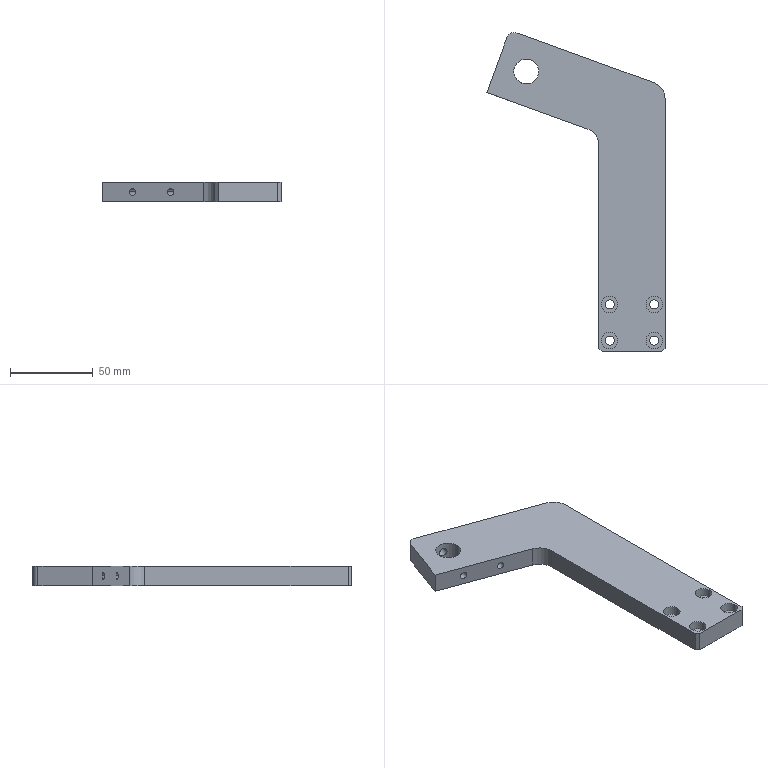Part | STEP file | 11-FG-B04911 | 1 solid | 45 faces | box 107.65 x 192.793 x 12 mm | volume 106173 mm3 | cylinder 27 | plane 14 | cone 4 | commonest cylinder face diameters 10 x9 5.5 x8 4.2 x4 5 x2 15.1 x2 20 x2
STEP:
#1=CARTESIAN_POINT('',(-47.528,162.486,6.));
#2=VERTEX_POINT('',#1);
#3=CARTESIAN_POINT('',(-43.582,161.05,6.));
#4=VERTEX_POINT('',#3);
#5=CARTESIAN_POINT('',(-45.555,161.768,6.));
#6=DIRECTION('',(-0.342,-0.9397,0.));
#7=DIRECTION('',(0.9397,-0.342,0.));
#8=AXIS2_PLACEMENT_3D('',#5,#6,#7);
#9=CIRCLE('',#8,2.1);
#10=EDGE_CURVE('',#2,#4,#9,.T.);
#11=ORIENTED_EDGE('',*,*,#10,.F.);
#12=CARTESIAN_POINT('',(-51.769,150.834,6.));
#13=VERTEX_POINT('',#12);
#14=CARTESIAN_POINT('',(-51.769,150.834,6.));
#15=DIRECTION('',(-0.342,-0.9397,0.));
#16=VECTOR('',#15,1000.);
#17=LINE('',#14,#16);
#18=EDGE_CURVE('',#2,#13,#17,.T.);
#19=ORIENTED_EDGE('',*,*,#18,.T.);
#20=CARTESIAN_POINT('',(-47.823,149.398,6.));
#21=VERTEX_POINT('',#20);
#22=CARTESIAN_POINT('',(-49.796,150.116,6.));
#23=DIRECTION('',(-0.342,-0.9397,0.));
#24=DIRECTION('',(0.9397,-0.342,0.));
#25=AXIS2_PLACEMENT_3D('',#22,#23,#24);
#26=CIRCLE('',#25,2.1);
#27=EDGE_CURVE('',#13,#21,#26,.T.);
#28=ORIENTED_EDGE('',*,*,#27,.T.);
#29=CARTESIAN_POINT('',(-47.823,149.398,6.));
#30=DIRECTION('',(-0.342,-0.9397,0.));
#31=VECTOR('',#30,1000.);
#32=LINE('',#29,#31);
#33=EDGE_CURVE('',#4,#21,#32,.T.);
#34=ORIENTED_EDGE('',*,*,#33,.F.);
#35=EDGE_LOOP('',(#11,#19,#28,#34));
#36=FACE_OUTER_BOUND('',#35,.T.);
#37=CARTESIAN_POINT('',(-49.796,150.116,6.));
#38=DIRECTION('',(-0.342,-0.9397,0.));
#39=DIRECTION('',(0.9397,-0.342,0.));
#40=AXIS2_PLACEMENT_3D('',#37,#38,#39);
#41=CYLINDRICAL_SURFACE('',#40,2.1);
#42=ADVANCED_FACE('',(#36),#41,.F.);
#43=CARTESIAN_POINT('',(-47.325,162.526,6.));
#44=VERTEX_POINT('',#43);
#45=CARTESIAN_POINT('',(-44.112,161.705,6.));
#46=VERTEX_POINT('',#45);
#47=CARTESIAN_POINT('',(-47.325,162.526,6.));
#48=CARTESIAN_POINT('',(-47.325,162.526,5.882));
#49=CARTESIAN_POINT('',(-47.317,162.522,5.765));
#50=CARTESIAN_POINT('',(-47.285,162.505,5.532));
#51=CARTESIAN_POINT('',(-47.26,162.493,5.416));
#52=CARTESIAN_POINT('',(-47.162,162.445,5.078));
#53=CARTESIAN_POINT('',(-47.065,162.398,4.868));
#54=CARTESIAN_POINT('',(-46.865,162.31,4.586));
#55=CARTESIAN_POINT('',(-46.791,162.279,4.5));
#56=CARTESIAN_POINT('',(-46.625,162.212,4.347));
#57=CARTESIAN_POINT('',(-46.532,162.177,4.278));
#58=CARTESIAN_POINT('',(-46.336,162.106,4.169));
#59=CARTESIAN_POINT('',(-46.232,162.072,4.127));
#60=CARTESIAN_POINT('',(-46.013,162.004,4.071));
#61=CARTESIAN_POINT('',(-45.898,161.971,4.058));
#62=CARTESIAN_POINT('',(-45.671,161.913,4.063));
#63=CARTESIAN_POINT('',(-45.555,161.886,4.081));
#64=CARTESIAN_POINT('',(-45.332,161.839,4.143));
#65=CARTESIAN_POINT('',(-45.223,161.819,4.188));
#66=CARTESIAN_POINT('',(-44.914,161.768,4.357));
#67=CARTESIAN_POINT('',(-44.731,161.747,4.513));
#68=CARTESIAN_POINT('',(-44.432,161.719,4.876));
#69=CARTESIAN_POINT('',(-44.313,161.713,5.086));
#70=CARTESIAN_POINT('',(-44.154,161.706,5.528));
#71=CARTESIAN_POINT('',(-44.112,161.705,5.765));
#72=CARTESIAN_POINT('',(-44.112,161.705,6.));
#73=B_SPLINE_CURVE_WITH_KNOTS('',3,(#47,#48,#49,#50,#51,#52,#53,#54,#55,#56,#57,#58,#59,#60,#61,#62,#63,#64,#65,#66,#67,#68,#69,#70,#71,#72),.UNSPECIFIED.,.F.,.F.,(4,2,2,2,2,2,2,2,2,2,2,2,4),(0.009239,0.00959,0.009941,0.01064,0.01099,0.01135,0.0117,0.01205,0.0124,0.01275,0.01345,0.01415,0.01486),.UNSPECIFIED.);
#74=EDGE_CURVE('',#44,#46,#73,.T.);
#75=ORIENTED_EDGE('',*,*,#74,.F.);
#76=CARTESIAN_POINT('',(-47.528,162.486,6.));
#77=DIRECTION('',(-0.9816,-0.1908,0.));
#78=VECTOR('',#77,1000.);
#79=LINE('',#76,#78);
#80=EDGE_CURVE('',#44,#2,#79,.T.);
#81=ORIENTED_EDGE('',*,*,#80,.T.);
#82=ORIENTED_EDGE('',*,*,#10,.T.);
#83=CARTESIAN_POINT('',(-43.582,161.05,6.));
#84=DIRECTION('',(0.6293,-0.7771,0.));
#85=VECTOR('',#84,1000.);
#86=LINE('',#83,#85);
#87=EDGE_CURVE('',#46,#4,#86,.T.);
#88=ORIENTED_EDGE('',*,*,#87,.F.);
#89=EDGE_LOOP('',(#75,#81,#82,#88));
#90=FACE_OUTER_BOUND('',#89,.T.);
#91=CARTESIAN_POINT('',(-45.555,161.768,6.));
#92=DIRECTION('',(-0.342,-0.9397,0.));
#93=DIRECTION('',(0.9397,-0.342,0.));
#94=AXIS2_PLACEMENT_3D('',#91,#92,#93);
#95=CONICAL_SURFACE('',#94,2.1,1.03);
#96=ADVANCED_FACE('',(#90),#95,.F.);
#97=CARTESIAN_POINT('',(-24.506,154.107,6.));
#98=VERTEX_POINT('',#97);
#99=CARTESIAN_POINT('',(-20.559,152.67,6.));
#100=VERTEX_POINT('',#99);
#101=CARTESIAN_POINT('',(-22.532,153.389,6.));
#102=DIRECTION('',(-0.342,-0.9397,0.));
#103=DIRECTION('',(0.9397,-0.342,0.));
#104=AXIS2_PLACEMENT_3D('',#101,#102,#103);
#105=CIRCLE('',#104,2.1);
#106=EDGE_CURVE('',#98,#100,#105,.T.);
#107=ORIENTED_EDGE('',*,*,#106,.F.);
#108=CARTESIAN_POINT('',(-28.747,142.455,6.));
#109=VERTEX_POINT('',#108);
#110=CARTESIAN_POINT('',(-28.747,142.455,6.));
#111=DIRECTION('',(-0.342,-0.9397,0.));
#112=VECTOR('',#111,1000.);
#113=LINE('',#110,#112);
#114=EDGE_CURVE('',#98,#109,#113,.T.);
#115=ORIENTED_EDGE('',*,*,#114,.T.);
#116=CARTESIAN_POINT('',(-24.8,141.018,6.));
#117=VERTEX_POINT('',#116);
#118=CARTESIAN_POINT('',(-26.773,141.736,6.));
#119=DIRECTION('',(-0.342,-0.9397,0.));
#120=DIRECTION('',(0.9397,-0.342,0.));
#121=AXIS2_PLACEMENT_3D('',#118,#119,#120);
#122=CIRCLE('',#121,2.1);
#123=EDGE_CURVE('',#109,#117,#122,.T.);
#124=ORIENTED_EDGE('',*,*,#123,.T.);
#125=CARTESIAN_POINT('',(-24.8,141.018,6.));
#126=DIRECTION('',(-0.342,-0.9397,0.));
#127=VECTOR('',#126,1000.);
#128=LINE('',#125,#127);
#129=EDGE_CURVE('',#100,#117,#128,.T.);
#130=ORIENTED_EDGE('',*,*,#129,.F.);
#131=EDGE_LOOP('',(#107,#115,#124,#130));
#132=FACE_OUTER_BOUND('',#131,.T.);
#133=CARTESIAN_POINT('',(-26.773,141.736,6.));
#134=DIRECTION('',(-0.342,-0.9397,0.));
#135=DIRECTION('',(0.9397,-0.342,0.));
#136=AXIS2_PLACEMENT_3D('',#133,#134,#135);
#137=CYLINDRICAL_SURFACE('',#136,2.1);
#138=ADVANCED_FACE('',(#132),#137,.F.);
#139=CARTESIAN_POINT('',(-22.101,154.574,6.));
#140=VERTEX_POINT('',#139);
#141=CARTESIAN_POINT('',(-20.559,152.67,6.));
#142=DIRECTION('',(0.6293,-0.7771,0.));
#143=VECTOR('',#142,1000.);
#144=LINE('',#141,#143);
#145=EDGE_CURVE('',#140,#100,#144,.T.);
#146=ORIENTED_EDGE('',*,*,#145,.F.);
#147=CARTESIAN_POINT('',(-24.506,154.107,6.));
#148=DIRECTION('',(-0.9816,-0.1908,0.));
#149=VECTOR('',#148,1000.);
#150=LINE('',#147,#149);
#151=EDGE_CURVE('',#140,#98,#150,.T.);
#152=ORIENTED_EDGE('',*,*,#151,.T.);
#153=ORIENTED_EDGE('',*,*,#106,.T.);
#154=EDGE_LOOP('',(#146,#152,#153));
#155=FACE_OUTER_BOUND('',#154,.T.);
#156=CARTESIAN_POINT('',(-22.532,153.389,6.));
#157=DIRECTION('',(-0.342,-0.9397,0.));
#158=DIRECTION('',(0.9397,-0.342,0.));
#159=AXIS2_PLACEMENT_3D('',#156,#157,#158);
#160=CONICAL_SURFACE('',#159,2.1,1.03);
#161=ADVANCED_FACE('',(#155),#160,.F.);
#162=CARTESIAN_POINT('',(-39.109,175.091,6.));
#163=VERTEX_POINT('',#162);
#164=CARTESIAN_POINT('',(-43.808,176.801,6.));
#165=VERTEX_POINT('',#164);
#166=CARTESIAN_POINT('',(-39.109,175.091,6.));
#167=CARTESIAN_POINT('',(-39.109,175.091,5.836));
#168=CARTESIAN_POINT('',(-39.123,175.102,5.671));
#169=CARTESIAN_POINT('',(-39.176,175.145,5.347));
#170=CARTESIAN_POINT('',(-39.216,175.177,5.191));
#171=CARTESIAN_POINT('',(-39.32,175.258,4.889));
#172=CARTESIAN_POINT('',(-39.385,175.307,4.743));
#173=CARTESIAN_POINT('',(-39.537,175.418,4.473));
#174=CARTESIAN_POINT('',(-39.624,175.479,4.348));
#175=CARTESIAN_POINT('',(-39.921,175.676,4.001));
#176=CARTESIAN_POINT('',(-40.159,175.82,3.818));
#177=CARTESIAN_POINT('',(-40.568,176.031,3.629));
#178=CARTESIAN_POINT('',(-40.709,176.099,3.581));
#179=CARTESIAN_POINT('',(-41.004,176.228,3.517));
#180=CARTESIAN_POINT('',(-41.158,176.29,3.5));
#181=CARTESIAN_POINT('',(-41.468,176.403,3.5));
#182=CARTESIAN_POINT('',(-41.623,176.454,3.516));
#183=CARTESIAN_POINT('',(-41.934,176.544,3.581));
#184=CARTESIAN_POINT('',(-42.089,176.584,3.629));
#185=CARTESIAN_POINT('',(-42.533,176.684,3.817));
#186=CARTESIAN_POINT('',(-42.812,176.727,4.003));
#187=CARTESIAN_POINT('',(-43.163,176.767,4.347));
#188=CARTESIAN_POINT('',(-43.271,176.777,4.475));
#189=CARTESIAN_POINT('',(-43.459,176.79,4.745));
#190=CARTESIAN_POINT('',(-43.539,176.794,4.888));
#191=CARTESIAN_POINT('',(-43.671,176.799,5.19));
#192=CARTESIAN_POINT('',(-43.722,176.8,5.349));
#193=CARTESIAN_POINT('',(-43.79,176.801,5.67));
#194=CARTESIAN_POINT('',(-43.808,176.801,5.834));
#195=CARTESIAN_POINT('',(-43.808,176.801,6.));
#196=B_SPLINE_CURVE_WITH_KNOTS('',3,(#166,#167,#168,#169,#170,#171,#172,#173,#174,#175,#176,#177,#178,#179,#180,#181,#182,#183,#184,#185,#186,#187,#188,#189,#190,#191,#192,#193,#194,#195),.UNSPECIFIED.,.F.,.F.,(4,2,2,2,2,2,2,2,2,2,2,2,2,2,4),(0.007872,0.008364,0.008856,0.009348,0.009839,0.01082,0.01131,0.01181,0.0123,0.01279,0.01377,0.01427,0.01476,0.01525,0.01574),.UNSPECIFIED.);
#197=EDGE_CURVE('',#163,#165,#196,.T.);
#198=ORIENTED_EDGE('',*,*,#197,.F.);
#199=CARTESIAN_POINT('',(-34.706,187.191,6.));
#200=VERTEX_POINT('',#199);
#201=CARTESIAN_POINT('',(-34.706,187.191,6.));
#202=DIRECTION('',(0.342,0.9397,0.));
#203=VECTOR('',#202,1000.);
#204=LINE('',#201,#203);
#205=EDGE_CURVE('',#163,#200,#204,.T.);
#206=ORIENTED_EDGE('',*,*,#205,.T.);
#207=CARTESIAN_POINT('',(-39.404,188.901,6.));
#208=VERTEX_POINT('',#207);
#209=CARTESIAN_POINT('',(-37.055,188.046,6.));
#210=DIRECTION('',(0.342,0.9397,0.));
#211=DIRECTION('',(-0.9397,0.342,0.));
#212=AXIS2_PLACEMENT_3D('',#209,#210,#211);
#213=CIRCLE('',#212,2.5);
#214=EDGE_CURVE('',#200,#208,#213,.T.);
#215=ORIENTED_EDGE('',*,*,#214,.T.);
#216=CARTESIAN_POINT('',(-39.404,188.901,6.));
#217=DIRECTION('',(0.342,0.9397,0.));
#218=VECTOR('',#217,1000.);
#219=LINE('',#216,#218);
#220=EDGE_CURVE('',#165,#208,#219,.T.);
#221=ORIENTED_EDGE('',*,*,#220,.F.);
#222=EDGE_LOOP('',(#198,#206,#215,#221));
#223=FACE_OUTER_BOUND('',#222,.T.);
#224=CARTESIAN_POINT('',(-37.055,188.046,6.));
#225=DIRECTION('',(0.342,0.9397,0.));
#226=DIRECTION('',(-0.9397,0.342,0.));
#227=AXIS2_PLACEMENT_3D('',#224,#225,#226);
#228=CYLINDRICAL_SURFACE('',#227,2.5);
#229=ADVANCED_FACE('',(#223),#228,.F.);
#230=CARTESIAN_POINT('',(1.5,28.5,6.6));
#231=VERTEX_POINT('',#230);
#232=CARTESIAN_POINT('',(11.5,28.5,6.6));
#233=VERTEX_POINT('',#232);
#234=CARTESIAN_POINT('',(6.5,28.5,6.6));
#235=DIRECTION('',(0.,0.,1.));
#236=DIRECTION('',(1.,0.,0.));
#237=AXIS2_PLACEMENT_3D('',#234,#235,#236);
#238=CIRCLE('',#237,5.);
#239=EDGE_CURVE('',#231,#233,#238,.T.);
#240=ORIENTED_EDGE('',*,*,#239,.F.);
#241=CARTESIAN_POINT('',(1.5,28.5,12.));
#242=VERTEX_POINT('',#241);
#243=CARTESIAN_POINT('',(1.5,28.5,12.));
#244=DIRECTION('',(0.,0.,1.));
#245=VECTOR('',#244,1000.);
#246=LINE('',#243,#245);
#247=EDGE_CURVE('',#231,#242,#246,.T.);
#248=ORIENTED_EDGE('',*,*,#247,.T.);
#249=CARTESIAN_POINT('',(11.5,28.5,12.));
#250=VERTEX_POINT('',#249);
#251=CARTESIAN_POINT('',(6.5,28.5,12.));
#252=DIRECTION('',(0.,0.,1.));
#253=DIRECTION('',(1.,0.,0.));
#254=AXIS2_PLACEMENT_3D('',#251,#252,#253);
#255=CIRCLE('',#254,5.);
#256=EDGE_CURVE('',#242,#250,#255,.T.);
#257=ORIENTED_EDGE('',*,*,#256,.T.);
#258=CARTESIAN_POINT('',(11.5,28.5,12.));
#259=DIRECTION('',(0.,0.,1.));
#260=VECTOR('',#259,1000.);
#261=LINE('',#258,#260);
#262=EDGE_CURVE('',#233,#250,#261,.T.);
#263=ORIENTED_EDGE('',*,*,#262,.F.);
#264=EDGE_LOOP('',(#240,#248,#257,#263));
#265=FACE_OUTER_BOUND('',#264,.T.);
#266=CARTESIAN_POINT('',(6.5,28.5,12.));
#267=DIRECTION('',(0.,0.,1.));
#268=DIRECTION('',(1.,0.,0.));
#269=AXIS2_PLACEMENT_3D('',#266,#267,#268);
#270=CYLINDRICAL_SURFACE('',#269,5.);
#271=ADVANCED_FACE('',(#265),#270,.F.);
#272=CARTESIAN_POINT('',(3.75,28.5,0.));
#273=VERTEX_POINT('',#272);
#274=CARTESIAN_POINT('',(9.25,28.5,0.));
#275=VERTEX_POINT('',#274);
#276=CARTESIAN_POINT('',(6.5,28.5,0.));
#277=DIRECTION('',(0.,0.,1.));
#278=DIRECTION('',(1.,0.,0.));
#279=AXIS2_PLACEMENT_3D('',#276,#277,#278);
#280=CIRCLE('',#279,2.75);
#281=EDGE_CURVE('',#273,#275,#280,.T.);
#282=ORIENTED_EDGE('',*,*,#281,.F.);
#283=CARTESIAN_POINT('',(3.75,28.5,6.6));
#284=VERTEX_POINT('',#283);
#285=CARTESIAN_POINT('',(3.75,28.5,12.));
#286=DIRECTION('',(0.,0.,1.));
#287=VECTOR('',#286,1000.);
#288=LINE('',#285,#287);
#289=EDGE_CURVE('',#273,#284,#288,.T.);
#290=ORIENTED_EDGE('',*,*,#289,.T.);
#291=CARTESIAN_POINT('',(9.25,28.5,6.6));
#292=VERTEX_POINT('',#291);
#293=CARTESIAN_POINT('',(6.5,28.5,6.6));
#294=DIRECTION('',(0.,0.,1.));
#295=DIRECTION('',(1.,0.,0.));
#296=AXIS2_PLACEMENT_3D('',#293,#294,#295);
#297=CIRCLE('',#296,2.75);
#298=EDGE_CURVE('',#284,#292,#297,.T.);
#299=ORIENTED_EDGE('',*,*,#298,.T.);
#300=CARTESIAN_POINT('',(9.25,28.5,12.));
#301=DIRECTION('',(0.,0.,1.));
#302=VECTOR('',#301,1000.);
#303=LINE('',#300,#302);
#304=EDGE_CURVE('',#275,#292,#303,.T.);
#305=ORIENTED_EDGE('',*,*,#304,.F.);
#306=EDGE_LOOP('',(#282,#290,#299,#305));
#307=FACE_OUTER_BOUND('',#306,.T.);
#308=CARTESIAN_POINT('',(6.5,28.5,12.));
#309=DIRECTION('',(0.,0.,1.));
#310=DIRECTION('',(1.,0.,0.));
#311=AXIS2_PLACEMENT_3D('',#308,#309,#310);
#312=CYLINDRICAL_SURFACE('',#311,2.75);
#313=ADVANCED_FACE('',(#307),#312,.F.);
#314=CARTESIAN_POINT('',(28.5,28.5,6.6));
#315=VERTEX_POINT('',#314);
#316=CARTESIAN_POINT('',(38.5,28.5,6.6));
#317=VERTEX_POINT('',#316);
#318=CARTESIAN_POINT('',(33.5,28.5,6.6));
#319=DIRECTION('',(0.,0.,1.));
#320=DIRECTION('',(1.,0.,0.));
#321=AXIS2_PLACEMENT_3D('',#318,#319,#320);
#322=CIRCLE('',#321,5.);
#323=EDGE_CURVE('',#315,#317,#322,.T.);
#324=ORIENTED_EDGE('',*,*,#323,.F.);
#325=CARTESIAN_POINT('',(28.5,28.5,12.));
#326=VERTEX_POINT('',#325);
#327=CARTESIAN_POINT('',(28.5,28.5,12.));
#328=DIRECTION('',(0.,0.,1.));
#329=VECTOR('',#328,1000.);
#330=LINE('',#327,#329);
#331=EDGE_CURVE('',#315,#326,#330,.T.);
#332=ORIENTED_EDGE('',*,*,#331,.T.);
#333=CARTESIAN_POINT('',(38.5,28.5,12.));
#334=VERTEX_POINT('',#333);
#335=CARTESIAN_POINT('',(33.5,28.5,12.));
#336=DIRECTION('',(0.,0.,1.));
#337=DIRECTION('',(1.,0.,0.));
#338=AXIS2_PLACEMENT_3D('',#335,#336,#337);
#339=CIRCLE('',#338,5.);
#340=EDGE_CURVE('',#326,#334,#339,.T.);
#341=ORIENTED_EDGE('',*,*,#340,.T.);
#342=CARTESIAN_POINT('',(38.5,28.5,12.));
#343=DIRECTION('',(0.,0.,1.));
#344=VECTOR('',#343,1000.);
#345=LINE('',#342,#344);
#346=EDGE_CURVE('',#317,#334,#345,.T.);
#347=ORIENTED_EDGE('',*,*,#346,.F.);
#348=EDGE_LOOP('',(#324,#332,#341,#347));
#349=FACE_OUTER_BOUND('',#348,.T.);
#350=CARTESIAN_POINT('',(33.5,28.5,12.));
#351=DIRECTION('',(0.,0.,1.));
#352=DIRECTION('',(1.,0.,0.));
#353=AXIS2_PLACEMENT_3D('',#350,#351,#352);
#354=CYLINDRICAL_SURFACE('',#353,5.);
#355=ADVANCED_FACE('',(#349),#354,.F.);
#356=CARTESIAN_POINT('',(30.75,28.5,0.));
#357=VERTEX_POINT('',#356);
#358=CARTESIAN_POINT('',(36.25,28.5,0.));
#359=VERTEX_POINT('',#358);
#360=CARTESIAN_POINT('',(33.5,28.5,0.));
#361=DIRECTION('',(0.,0.,1.));
#362=DIRECTION('',(1.,0.,0.));
#363=AXIS2_PLACEMENT_3D('',#360,#361,#362);
#364=CIRCLE('',#363,2.75);
#365=EDGE_CURVE('',#357,#359,#364,.T.);
#366=ORIENTED_EDGE('',*,*,#365,.F.);
#367=CARTESIAN_POINT('',(30.75,28.5,6.6));
#368=VERTEX_POINT('',#367);
#369=CARTESIAN_POINT('',(30.75,28.5,12.));
#370=DIRECTION('',(0.,0.,1.));
#371=VECTOR('',#370,1000.);
#372=LINE('',#369,#371);
#373=EDGE_CURVE('',#357,#368,#372,.T.);
#374=ORIENTED_EDGE('',*,*,#373,.T.);
#375=CARTESIAN_POINT('',(36.25,28.5,6.6));
#376=VERTEX_POINT('',#375);
#377=CARTESIAN_POINT('',(33.5,28.5,6.6));
#378=DIRECTION('',(0.,0.,1.));
#379=DIRECTION('',(1.,0.,0.));
#380=AXIS2_PLACEMENT_3D('',#377,#378,#379);
#381=CIRCLE('',#380,2.75);
#382=EDGE_CURVE('',#368,#376,#381,.T.);
#383=ORIENTED_EDGE('',*,*,#382,.T.);
#384=CARTESIAN_POINT('',(36.25,28.5,12.));
#385=DIRECTION('',(0.,0.,1.));
#386=VECTOR('',#385,1000.);
#387=LINE('',#384,#386);
#388=EDGE_CURVE('',#359,#376,#387,.T.);
#389=ORIENTED_EDGE('',*,*,#388,.F.);
#390=EDGE_LOOP('',(#366,#374,#383,#389));
#391=FACE_OUTER_BOUND('',#390,.T.);
#392=CARTESIAN_POINT('',(33.5,28.5,12.));
#393=DIRECTION('',(0.,0.,1.));
#394=DIRECTION('',(1.,0.,0.));
#395=AXIS2_PLACEMENT_3D('',#392,#393,#394);
#396=CYLINDRICAL_SURFACE('',#395,2.75);
#397=ADVANCED_FACE('',(#391),#396,.F.);
#398=CARTESIAN_POINT('',(1.5,6.5,6.6));
#399=VERTEX_POINT('',#398);
#400=CARTESIAN_POINT('',(11.5,6.5,6.6));
#401=VERTEX_POINT('',#400);
#402=CARTESIAN_POINT('',(6.5,6.5,6.6));
#403=DIRECTION('',(0.,0.,1.));
#404=DIRECTION('',(1.,0.,0.));
#405=AXIS2_PLACEMENT_3D('',#402,#403,#404);
#406=CIRCLE('',#405,5.);
#407=EDGE_CURVE('',#399,#401,#406,.T.);
#408=ORIENTED_EDGE('',*,*,#407,.F.);
#409=CARTESIAN_POINT('',(1.5,6.5,12.));
#410=VERTEX_POINT('',#409);
#411=CARTESIAN_POINT('',(1.5,6.5,12.));
#412=DIRECTION('',(0.,0.,1.));
#413=VECTOR('',#412,1000.);
#414=LINE('',#411,#413);
#415=EDGE_CURVE('',#399,#410,#414,.T.);
#416=ORIENTED_EDGE('',*,*,#415,.T.);
#417=CARTESIAN_POINT('',(11.5,6.5,12.));
#418=VERTEX_POINT('',#417);
#419=CARTESIAN_POINT('',(6.5,6.5,12.));
#420=DIRECTION('',(0.,0.,1.));
#421=DIRECTION('',(1.,0.,0.));
#422=AXIS2_PLACEMENT_3D('',#419,#420,#421);
#423=CIRCLE('',#422,5.);
#424=EDGE_CURVE('',#410,#418,#423,.T.);
#425=ORIENTED_EDGE('',*,*,#424,.T.);
#426=CARTESIAN_POINT('',(11.5,6.5,12.));
#427=DIRECTION('',(0.,0.,1.));
#428=VECTOR('',#427,1000.);
#429=LINE('',#426,#428);
#430=EDGE_CURVE('',#401,#418,#429,.T.);
#431=ORIENTED_EDGE('',*,*,#430,.F.);
#432=EDGE_LOOP('',(#408,#416,#425,#431));
#433=FACE_OUTER_BOUND('',#432,.T.);
#434=CARTESIAN_POINT('',(6.5,6.5,12.));
#435=DIRECTION('',(0.,0.,1.));
#436=DIRECTION('',(1.,0.,0.));
#437=AXIS2_PLACEMENT_3D('',#434,#435,#436);
#438=CYLINDRICAL_SURFACE('',#437,5.);
#439=ADVANCED_FACE('',(#433),#438,.F.);
#440=CARTESIAN_POINT('',(3.75,6.5,0.));
#441=VERTEX_POINT('',#440);
#442=CARTESIAN_POINT('',(9.25,6.5,0.));
#443=VERTEX_POINT('',#442);
#444=CARTESIAN_POINT('',(6.5,6.5,0.));
#445=DIRECTION('',(0.,0.,1.));
#446=DIRECTION('',(1.,0.,0.));
#447=AXIS2_PLACEMENT_3D('',#444,#445,#446);
#448=CIRCLE('',#447,2.75);
#449=EDGE_CURVE('',#441,#443,#448,.T.);
#450=ORIENTED_EDGE('',*,*,#449,.F.);
#451=CARTESIAN_POINT('',(3.75,6.5,6.6));
#452=VERTEX_POINT('',#451);
#453=CARTESIAN_POINT('',(3.75,6.5,12.));
#454=DIRECTION('',(0.,0.,1.));
#455=VECTOR('',#454,1000.);
#456=LINE('',#453,#455);
#457=EDGE_CURVE('',#441,#452,#456,.T.);
#458=ORIENTED_EDGE('',*,*,#457,.T.);
#459=CARTESIAN_POINT('',(9.25,6.5,6.6));
#460=VERTEX_POINT('',#459);
#461=CARTESIAN_POINT('',(6.5,6.5,6.6));
#462=DIRECTION('',(0.,0.,1.));
#463=DIRECTION('',(1.,0.,0.));
#464=AXIS2_PLACEMENT_3D('',#461,#462,#463);
#465=CIRCLE('',#464,2.75);
#466=EDGE_CURVE('',#452,#460,#465,.T.);
#467=ORIENTED_EDGE('',*,*,#466,.T.);
#468=CARTESIAN_POINT('',(9.25,6.5,12.));
#469=DIRECTION('',(0.,0.,1.));
#470=VECTOR('',#469,1000.);
#471=LINE('',#468,#470);
#472=EDGE_CURVE('',#443,#460,#471,.T.);
#473=ORIENTED_EDGE('',*,*,#472,.F.);
#474=EDGE_LOOP('',(#450,#458,#467,#473));
#475=FACE_OUTER_BOUND('',#474,.T.);
#476=CARTESIAN_POINT('',(6.5,6.5,12.));
#477=DIRECTION('',(0.,0.,1.));
#478=DIRECTION('',(1.,0.,0.));
#479=AXIS2_PLACEMENT_3D('',#476,#477,#478);
#480=CYLINDRICAL_SURFACE('',#479,2.75);
#481=ADVANCED_FACE('',(#475),#480,.F.);
#482=CARTESIAN_POINT('',(28.5,6.5,6.6));
#483=VERTEX_POINT('',#482);
#484=CARTESIAN_POINT('',(38.5,6.5,6.6));
#485=VERTEX_POINT('',#484);
#486=CARTESIAN_POINT('',(33.5,6.5,6.6));
#487=DIRECTION('',(0.,0.,1.));
#488=DIRECTION('',(1.,0.,0.));
#489=AXIS2_PLACEMENT_3D('',#486,#487,#488);
#490=CIRCLE('',#489,5.);
#491=EDGE_CURVE('',#483,#485,#490,.T.);
#492=ORIENTED_EDGE('',*,*,#491,.F.);
#493=CARTESIAN_POINT('',(28.5,6.5,12.));
#494=VERTEX_POINT('',#493);
#495=CARTESIAN_POINT('',(28.5,6.5,12.));
#496=DIRECTION('',(0.,0.,1.));
#497=VECTOR('',#496,1000.);
#498=LINE('',#495,#497);
#499=EDGE_CURVE('',#483,#494,#498,.T.);
#500=ORIENTED_EDGE('',*,*,#499,.T.);
#501=CARTESIAN_POINT('',(38.5,6.5,12.));
#502=VERTEX_POINT('',#501);
#503=CARTESIAN_POINT('',(33.5,6.5,12.));
#504=DIRECTION('',(0.,0.,1.));
#505=DIRECTION('',(1.,0.,0.));
#506=AXIS2_PLACEMENT_3D('',#503,#504,#505);
#507=CIRCLE('',#506,5.);
#508=EDGE_CURVE('',#494,#502,#507,.T.);
#509=ORIENTED_EDGE('',*,*,#508,.T.);
#510=CARTESIAN_POINT('',(38.5,6.5,12.));
#511=DIRECTION('',(0.,0.,1.));
#512=VECTOR('',#511,1000.);
#513=LINE('',#510,#512);
#514=EDGE_CURVE('',#485,#502,#513,.T.);
#515=ORIENTED_EDGE('',*,*,#514,.F.);
#516=EDGE_LOOP('',(#492,#500,#509,#515));
#517=FACE_OUTER_BOUND('',#516,.T.);
#518=CARTESIAN_POINT('',(33.5,6.5,12.));
#519=DIRECTION('',(0.,0.,1.));
#520=DIRECTION('',(1.,0.,0.));
#521=AXIS2_PLACEMENT_3D('',#518,#519,#520);
#522=CYLINDRICAL_SURFACE('',#521,5.);
#523=ADVANCED_FACE('',(#517),#522,.F.);
#524=CARTESIAN_POINT('',(30.75,6.5,0.));
#525=VERTEX_POINT('',#524);
#526=CARTESIAN_POINT('',(36.25,6.5,0.));
#527=VERTEX_POINT('',#526);
#528=CARTESIAN_POINT('',(33.5,6.5,0.));
#529=DIRECTION('',(0.,0.,1.));
#530=DIRECTION('',(1.,0.,0.));
#531=AXIS2_PLACEMENT_3D('',#528,#529,#530);
#532=CIRCLE('',#531,2.75);
#533=EDGE_CURVE('',#525,#527,#532,.T.);
#534=ORIENTED_EDGE('',*,*,#533,.F.);
#535=CARTESIAN_POINT('',(30.75,6.5,6.6));
#536=VERTEX_POINT('',#535);
#537=CARTESIAN_POINT('',(30.75,6.5,12.));
#538=DIRECTION('',(0.,0.,1.));
#539=VECTOR('',#538,1000.);
#540=LINE('',#537,#539);
#541=EDGE_CURVE('',#525,#536,#540,.T.);
#542=ORIENTED_EDGE('',*,*,#541,.T.);
#543=CARTESIAN_POINT('',(36.25,6.5,6.6));
#544=VERTEX_POINT('',#543);
#545=CARTESIAN_POINT('',(33.5,6.5,6.6));
#546=DIRECTION('',(0.,0.,1.));
#547=DIRECTION('',(1.,0.,0.));
#548=AXIS2_PLACEMENT_3D('',#545,#546,#547);
#549=CIRCLE('',#548,2.75);
#550=EDGE_CURVE('',#536,#544,#549,.T.);
#551=ORIENTED_EDGE('',*,*,#550,.T.);
#552=CARTESIAN_POINT('',(36.25,6.5,12.));
#553=DIRECTION('',(0.,0.,1.));
#554=VECTOR('',#553,1000.);
#555=LINE('',#552,#554);
#556=EDGE_CURVE('',#527,#544,#555,.T.);
#557=ORIENTED_EDGE('',*,*,#556,.F.);
#558=EDGE_LOOP('',(#534,#542,#551,#557));
#559=FACE_OUTER_BOUND('',#558,.T.);
#560=CARTESIAN_POINT('',(33.5,6.5,12.));
#561=DIRECTION('',(0.,0.,1.));
#562=DIRECTION('',(1.,0.,0.));
#563=AXIS2_PLACEMENT_3D('',#560,#561,#562);
#564=CYLINDRICAL_SURFACE('',#563,2.75);
#565=ADVANCED_FACE('',(#559),#564,.F.);
#566=CARTESIAN_POINT('',(-44.112,161.705,6.));
#567=CARTESIAN_POINT('',(-44.112,161.705,6.234));
#568=CARTESIAN_POINT('',(-44.154,161.706,6.472));
#569=CARTESIAN_POINT('',(-44.313,161.713,6.913));
#570=CARTESIAN_POINT('',(-44.431,161.719,7.123));
#571=CARTESIAN_POINT('',(-44.654,161.74,7.394));
#572=CARTESIAN_POINT('',(-44.738,161.748,7.479));
#573=CARTESIAN_POINT('',(-44.917,161.771,7.63));
#574=CARTESIAN_POINT('',(-45.013,161.784,7.696));
#575=CARTESIAN_POINT('',(-45.216,161.817,7.808));
#576=CARTESIAN_POINT('',(-45.325,161.838,7.854));
#577=CARTESIAN_POINT('',(-45.548,161.884,7.918));
#578=CARTESIAN_POINT('',(-45.661,161.91,7.936));
#579=CARTESIAN_POINT('',(-45.892,161.97,7.942));
#580=CARTESIAN_POINT('',(-46.005,162.002,7.93));
#581=CARTESIAN_POINT('',(-46.225,162.069,7.876));
#582=CARTESIAN_POINT('',(-46.332,162.105,7.833));
#583=CARTESIAN_POINT('',(-46.529,162.175,7.724));
#584=CARTESIAN_POINT('',(-46.621,162.211,7.657));
#585=CARTESIAN_POINT('',(-46.788,162.277,7.503));
#586=CARTESIAN_POINT('',(-46.863,162.309,7.417));
#587=CARTESIAN_POINT('',(-47.064,162.397,7.135));
#588=CARTESIAN_POINT('',(-47.162,162.445,6.922));
#589=CARTESIAN_POINT('',(-47.26,162.493,6.585));
#590=CARTESIAN_POINT('',(-47.284,162.505,6.47));
#591=CARTESIAN_POINT('',(-47.317,162.522,6.237));
#592=CARTESIAN_POINT('',(-47.325,162.526,6.118));
#593=CARTESIAN_POINT('',(-47.325,162.526,6.));
#594=B_SPLINE_CURVE_WITH_KNOTS('',3,(#566,#567,#568,#569,#570,#571,#572,#573,#574,#575,#576,#577,#578,#579,#580,#581,#582,#583,#584,#585,#586,#587,#588,#589,#590,#591,#592,#593),.UNSPECIFIED.,.F.,.F.,(4,2,2,2,2,2,2,2,2,2,2,2,2,4),(0.003628,0.004329,0.00503,0.005381,0.005732,0.006082,0.006433,0.006784,0.007134,0.007485,0.007836,0.008537,0.008888,0.009239),.UNSPECIFIED.);
#595=EDGE_CURVE('',#46,#44,#594,.T.);
#596=ORIENTED_EDGE('',*,*,#595,.T.);
#597=ORIENTED_EDGE('',*,*,#74,.T.);
#598=EDGE_LOOP('',(#596,#597));
#599=FACE_BOUND('',#598,.T.);
#600=CARTESIAN_POINT('',(-36.345,169.252,0.));
#601=VERTEX_POINT('',#600);
#602=CARTESIAN_POINT('',(-51.445,169.252,0.));
#603=VERTEX_POINT('',#602);
#604=CARTESIAN_POINT('',(-43.895,169.252,0.));
#605=DIRECTION('',(0.,0.,-1.));
#606=DIRECTION('',(-1.,0.,0.));
#607=AXIS2_PLACEMENT_3D('',#604,#605,#606);
#608=CIRCLE('',#607,7.55);
#609=EDGE_CURVE('',#601,#603,#608,.T.);
#610=ORIENTED_EDGE('',*,*,#609,.T.);
#611=CARTESIAN_POINT('',(-51.445,169.252,12.));
#612=VERTEX_POINT('',#611);
#613=CARTESIAN_POINT('',(-51.445,169.252,-27.));
#614=DIRECTION('',(0.,0.,1.));
#615=VECTOR('',#614,1000.);
#616=LINE('',#613,#615);
#617=EDGE_CURVE('',#603,#612,#616,.T.);
#618=ORIENTED_EDGE('',*,*,#617,.T.);
#619=CARTESIAN_POINT('',(-36.345,169.252,12.));
#620=VERTEX_POINT('',#619);
#621=CARTESIAN_POINT('',(-43.895,169.252,12.));
#622=DIRECTION('',(0.,0.,1.));
#623=DIRECTION('',(1.,0.,0.));
#624=AXIS2_PLACEMENT_3D('',#621,#622,#623);
#625=CIRCLE('',#624,7.55);
#626=EDGE_CURVE('',#612,#620,#625,.T.);
#627=ORIENTED_EDGE('',*,*,#626,.T.);
#628=CARTESIAN_POINT('',(-36.345,169.252,-27.));
#629=DIRECTION('',(0.,0.,1.));
#630=VECTOR('',#629,1000.);
#631=LINE('',#628,#630);
#632=EDGE_CURVE('',#601,#620,#631,.T.);
#633=ORIENTED_EDGE('',*,*,#632,.F.);
#634=EDGE_LOOP('',(#610,#618,#627,#633));
#635=FACE_OUTER_BOUND('',#634,.T.);
#636=CARTESIAN_POINT('',(-43.895,169.252,-27.));
#637=DIRECTION('',(0.,0.,1.));
#638=DIRECTION('',(1.,0.,0.));
#639=AXIS2_PLACEMENT_3D('',#636,#637,#638);
#640=CYLINDRICAL_SURFACE('',#639,7.55);
#641=ADVANCED_FACE('',(#599,#635),#640,.F.);
#642=CARTESIAN_POINT('',(0.,124.99,0.));
#643=VERTEX_POINT('',#642);
#644=CARTESIAN_POINT('',(0.,2.,0.));
#645=VERTEX_POINT('',#644);
#646=CARTESIAN_POINT('',(0.,0.,0.));
#647=DIRECTION('',(0.,-1.,0.));
#648=VECTOR('',#647,1000.);
#649=LINE('',#646,#648);
#650=EDGE_CURVE('',#643,#645,#649,.T.);
#651=ORIENTED_EDGE('',*,*,#650,.T.);
#652=CARTESIAN_POINT('',(0.,2.,12.));
#653=VERTEX_POINT('',#652);
#654=CARTESIAN_POINT('',(0.,2.,12.));
#655=DIRECTION('',(0.,0.,1.));
#656=VECTOR('',#655,1000.);
#657=LINE('',#654,#656);
#658=EDGE_CURVE('',#645,#653,#657,.T.);
#659=ORIENTED_EDGE('',*,*,#658,.T.);
#660=CARTESIAN_POINT('',(0.,124.99,12.));
#661=VERTEX_POINT('',#660);
#662=CARTESIAN_POINT('',(0.,0.,12.));
#663=DIRECTION('',(0.,-1.,0.));
#664=VECTOR('',#663,1000.);
#665=LINE('',#662,#664);
#666=EDGE_CURVE('',#661,#653,#665,.T.);
#667=ORIENTED_EDGE('',*,*,#666,.F.);
#668=CARTESIAN_POINT('',(0.,124.99,0.));
#669=DIRECTION('',(0.,0.,-1.));
#670=VECTOR('',#669,1000.);
#671=LINE('',#668,#670);
#672=EDGE_CURVE('',#661,#643,#671,.T.);
#673=ORIENTED_EDGE('',*,*,#672,.T.);
#674=EDGE_LOOP('',(#651,#659,#667,#673));
#675=FACE_OUTER_BOUND('',#674,.T.);
#676=CARTESIAN_POINT('',(0.,0.,12.));
#677=DIRECTION('',(1.,0.,0.));
#678=DIRECTION('',(0.,1.,0.));
#679=AXIS2_PLACEMENT_3D('',#676,#677,#678);
#680=PLANE('',#679);
#681=ADVANCED_FACE('',(#675),#680,.F.);
#682=CARTESIAN_POINT('',(2.,0.,0.));
#683=VERTEX_POINT('',#682);
#684=CARTESIAN_POINT('',(38.,0.,0.));
#685=VERTEX_POINT('',#684);
#686=CARTESIAN_POINT('',(0.,0.,0.));
#687=DIRECTION('',(1.,0.,0.));
#688=VECTOR('',#687,1000.);
#689=LINE('',#686,#688);
#690=EDGE_CURVE('',#683,#685,#689,.T.);
#691=ORIENTED_EDGE('',*,*,#690,.T.);
#692=CARTESIAN_POINT('',(38.,0.,12.));
#693=VERTEX_POINT('',#692);
#694=CARTESIAN_POINT('',(38.,0.,12.));
#695=DIRECTION('',(0.,0.,1.));
#696=VECTOR('',#695,1000.);
#697=LINE('',#694,#696);
#698=EDGE_CURVE('',#685,#693,#697,.T.);
#699=ORIENTED_EDGE('',*,*,#698,.T.);
#700=CARTESIAN_POINT('',(2.,0.,12.));
#701=VERTEX_POINT('',#700);
#702=CARTESIAN_POINT('',(0.,0.,12.));
#703=DIRECTION('',(1.,0.,0.));
#704=VECTOR('',#703,1000.);
#705=LINE('',#702,#704);
#706=EDGE_CURVE('',#701,#693,#705,.T.);
#707=ORIENTED_EDGE('',*,*,#706,.F.);
#708=CARTESIAN_POINT('',(2.,0.,12.));
#709=DIRECTION('',(0.,0.,-1.));
#710=VECTOR('',#709,1000.);
#711=LINE('',#708,#710);
#712=EDGE_CURVE('',#701,#683,#711,.T.);
#713=ORIENTED_EDGE('',*,*,#712,.T.);
#714=EDGE_LOOP('',(#691,#699,#707,#713));
#715=FACE_OUTER_BOUND('',#714,.T.);
#716=CARTESIAN_POINT('',(0.,0.,12.));
#717=DIRECTION('',(0.,1.,0.));
#718=DIRECTION('',(0.,0.,1.));
#719=AXIS2_PLACEMENT_3D('',#716,#717,#718);
#720=PLANE('',#719);
#721=ADVANCED_FACE('',(#715),#720,.F.);
#722=CARTESIAN_POINT('',(40.,2.,12.));
#723=VERTEX_POINT('',#722);
#724=CARTESIAN_POINT('',(40.,152.998,12.));
#725=VERTEX_POINT('',#724);
#726=CARTESIAN_POINT('',(40.,0.,12.));
#727=DIRECTION('',(0.,1.,0.));
#728=VECTOR('',#727,1000.);
#729=LINE('',#726,#728);
#730=EDGE_CURVE('',#723,#725,#729,.T.);
#731=ORIENTED_EDGE('',*,*,#730,.F.);
#732=CARTESIAN_POINT('',(40.,2.,0.));
#733=VERTEX_POINT('',#732);
#734=CARTESIAN_POINT('',(40.,2.,12.));
#735=DIRECTION('',(0.,0.,-1.));
#736=VECTOR('',#735,1000.);
#737=LINE('',#734,#736);
#738=EDGE_CURVE('',#723,#733,#737,.T.);
#739=ORIENTED_EDGE('',*,*,#738,.T.);
#740=CARTESIAN_POINT('',(40.,152.998,0.));
#741=VERTEX_POINT('',#740);
#742=CARTESIAN_POINT('',(40.,0.,0.));
#743=DIRECTION('',(0.,1.,0.));
#744=VECTOR('',#743,1000.);
#745=LINE('',#742,#744);
#746=EDGE_CURVE('',#733,#741,#745,.T.);
#747=ORIENTED_EDGE('',*,*,#746,.T.);
#748=CARTESIAN_POINT('',(40.,152.998,12.));
#749=DIRECTION('',(0.,0.,1.));
#750=VECTOR('',#749,1000.);
#751=LINE('',#748,#750);
#752=EDGE_CURVE('',#741,#725,#751,.T.);
#753=ORIENTED_EDGE('',*,*,#752,.T.);
#754=EDGE_LOOP('',(#731,#739,#747,#753));
#755=FACE_OUTER_BOUND('',#754,.T.);
#756=CARTESIAN_POINT('',(40.,0.,12.));
#757=DIRECTION('',(-1.,0.,0.));
#758=DIRECTION('',(0.,-1.,0.));
#759=AXIS2_PLACEMENT_3D('',#756,#757,#758);
#760=PLANE('',#759);
#761=ADVANCED_FACE('',(#755),#760,.F.);
#762=CARTESIAN_POINT('',(-37.055,188.046,6.));
#763=DIRECTION('',(0.342,0.9397,0.));
#764=DIRECTION('',(-0.9397,0.342,0.));
#765=AXIS2_PLACEMENT_3D('',#762,#763,#764);
#766=CIRCLE('',#765,2.5);
#767=EDGE_CURVE('',#208,#200,#766,.T.);
#768=ORIENTED_EDGE('',*,*,#767,.F.);
#769=ORIENTED_EDGE('',*,*,#214,.F.);
#770=EDGE_LOOP('',(#768,#769));
#771=FACE_BOUND('',#770,.T.);
#772=CARTESIAN_POINT('',(33.42,162.395,0.));
#773=VERTEX_POINT('',#772);
#774=CARTESIAN_POINT('',(-49.271,192.492,0.));
#775=VERTEX_POINT('',#774);
#776=CARTESIAN_POINT('',(40.,160.,0.));
#777=DIRECTION('',(-0.9397,0.342,0.));
#778=VECTOR('',#777,1000.);
#779=LINE('',#776,#778);
#780=EDGE_CURVE('',#773,#775,#779,.T.);
#781=ORIENTED_EDGE('',*,*,#780,.T.);
#782=CARTESIAN_POINT('',(-49.271,192.492,12.));
#783=VERTEX_POINT('',#782);
#784=CARTESIAN_POINT('',(-49.271,192.492,12.));
#785=DIRECTION('',(0.,0.,1.));
#786=VECTOR('',#785,1000.);
#787=LINE('',#784,#786);
#788=EDGE_CURVE('',#775,#783,#787,.T.);
#789=ORIENTED_EDGE('',*,*,#788,.T.);
#790=CARTESIAN_POINT('',(33.42,162.395,12.));
#791=VERTEX_POINT('',#790);
#792=CARTESIAN_POINT('',(40.,160.,12.));
#793=DIRECTION('',(-0.9397,0.342,0.));
#794=VECTOR('',#793,1000.);
#795=LINE('',#792,#794);
#796=EDGE_CURVE('',#791,#783,#795,.T.);
#797=ORIENTED_EDGE('',*,*,#796,.F.);
#798=CARTESIAN_POINT('',(33.42,162.395,12.));
#799=DIRECTION('',(0.,0.,-1.));
#800=VECTOR('',#799,1000.);
#801=LINE('',#798,#800);
#802=EDGE_CURVE('',#791,#773,#801,.T.);
#803=ORIENTED_EDGE('',*,*,#802,.T.);
#804=EDGE_LOOP('',(#781,#789,#797,#803));
#805=FACE_OUTER_BOUND('',#804,.T.);
#806=CARTESIAN_POINT('',(40.,160.,12.));
#807=DIRECTION('',(-0.342,-0.9397,0.));
#808=DIRECTION('',(0.9397,-0.342,0.));
#809=AXIS2_PLACEMENT_3D('',#806,#807,#808);
#810=PLANE('',#809);
#811=ADVANCED_FACE('',(#771,#805),#810,.F.);
#812=CARTESIAN_POINT('',(-55.679,189.504,12.));
#813=VERTEX_POINT('',#812);
#814=CARTESIAN_POINT('',(-67.65,156.614,12.));
#815=VERTEX_POINT('',#814);
#816=CARTESIAN_POINT('',(-53.969,194.202,12.));
#817=DIRECTION('',(-0.342,-0.9397,0.));
#818=VECTOR('',#817,1000.);
#819=LINE('',#816,#818);
#820=EDGE_CURVE('',#813,#815,#819,.T.);
#821=ORIENTED_EDGE('',*,*,#820,.F.);
#822=CARTESIAN_POINT('',(-55.679,189.504,0.));
#823=VERTEX_POINT('',#822);
#824=CARTESIAN_POINT('',(-55.679,189.504,12.));
#825=DIRECTION('',(0.,0.,-1.));
#826=VECTOR('',#825,1000.);
#827=LINE('',#824,#826);
#828=EDGE_CURVE('',#813,#823,#827,.T.);
#829=ORIENTED_EDGE('',*,*,#828,.T.);
#830=CARTESIAN_POINT('',(-67.65,156.614,0.));
#831=VERTEX_POINT('',#830);
#832=CARTESIAN_POINT('',(-53.969,194.202,0.));
#833=DIRECTION('',(-0.342,-0.9397,0.));
#834=VECTOR('',#833,1000.);
#835=LINE('',#832,#834);
#836=EDGE_CURVE('',#823,#831,#835,.T.);
#837=ORIENTED_EDGE('',*,*,#836,.T.);
#838=CARTESIAN_POINT('',(-67.65,156.614,12.));
#839=DIRECTION('',(0.,0.,-1.));
#840=VECTOR('',#839,1000.);
#841=LINE('',#838,#840);
#842=EDGE_CURVE('',#815,#831,#841,.T.);
#843=ORIENTED_EDGE('',*,*,#842,.F.);
#844=EDGE_LOOP('',(#821,#829,#837,#843));
#845=FACE_OUTER_BOUND('',#844,.T.);
#846=CARTESIAN_POINT('',(-53.969,194.202,12.));
#847=DIRECTION('',(0.9397,-0.342,0.));
#848=DIRECTION('',(0.342,0.9397,0.));
#849=AXIS2_PLACEMENT_3D('',#846,#847,#848);
#850=PLANE('',#849);
#851=ADVANCED_FACE('',(#845),#850,.F.);
#852=CARTESIAN_POINT('',(-49.796,150.116,6.));
#853=DIRECTION('',(-0.342,-0.9397,0.));
#854=DIRECTION('',(0.9397,-0.342,0.));
#855=AXIS2_PLACEMENT_3D('',#852,#853,#854);
#856=CIRCLE('',#855,2.1);
#857=EDGE_CURVE('',#21,#13,#856,.T.);
#858=ORIENTED_EDGE('',*,*,#857,.F.);
#859=ORIENTED_EDGE('',*,*,#27,.F.);
#860=EDGE_LOOP('',(#858,#859));
#861=FACE_BOUND('',#860,.T.);
#862=CARTESIAN_POINT('',(-26.773,141.736,6.));
#863=DIRECTION('',(-0.342,-0.9397,0.));
#864=DIRECTION('',(0.9397,-0.342,0.));
#865=AXIS2_PLACEMENT_3D('',#862,#863,#864);
#866=CIRCLE('',#865,2.1);
#867=EDGE_CURVE('',#117,#109,#866,.T.);
#868=ORIENTED_EDGE('',*,*,#867,.F.);
#869=ORIENTED_EDGE('',*,*,#123,.F.);
#870=EDGE_LOOP('',(#868,#869));
#871=FACE_BOUND('',#870,.T.);
#872=CARTESIAN_POINT('',(-6.58,134.387,0.));
#873=VERTEX_POINT('',#872);
#874=CARTESIAN_POINT('',(0.,131.992,0.));
#875=DIRECTION('',(0.9397,-0.342,0.));
#876=VECTOR('',#875,1000.);
#877=LINE('',#874,#876);
#878=EDGE_CURVE('',#831,#873,#877,.T.);
#879=ORIENTED_EDGE('',*,*,#878,.T.);
#880=CARTESIAN_POINT('',(-6.58,134.387,12.));
#881=VERTEX_POINT('',#880);
#882=CARTESIAN_POINT('',(-6.58,134.387,12.));
#883=DIRECTION('',(0.,0.,1.));
#884=VECTOR('',#883,1000.);
#885=LINE('',#882,#884);
#886=EDGE_CURVE('',#873,#881,#885,.T.);
#887=ORIENTED_EDGE('',*,*,#886,.T.);
#888=CARTESIAN_POINT('',(0.,131.992,12.));
#889=DIRECTION('',(0.9397,-0.342,0.));
#890=VECTOR('',#889,1000.);
#891=LINE('',#888,#890);
#892=EDGE_CURVE('',#815,#881,#891,.T.);
#893=ORIENTED_EDGE('',*,*,#892,.F.);
#894=ORIENTED_EDGE('',*,*,#842,.T.);
#895=EDGE_LOOP('',(#879,#887,#893,#894));
#896=FACE_OUTER_BOUND('',#895,.T.);
#897=CARTESIAN_POINT('',(0.,131.992,12.));
#898=DIRECTION('',(0.342,0.9397,0.));
#899=DIRECTION('',(-0.9397,0.342,0.));
#900=AXIS2_PLACEMENT_3D('',#897,#898,#899);
#901=PLANE('',#900);
#902=ADVANCED_FACE('',(#861,#871,#896),#901,.F.);
#903=CARTESIAN_POINT('',(6.5,28.5,12.));
#904=DIRECTION('',(0.,0.,1.));
#905=DIRECTION('',(1.,0.,0.));
#906=AXIS2_PLACEMENT_3D('',#903,#904,#905);
#907=CIRCLE('',#906,5.);
#908=EDGE_CURVE('',#250,#242,#907,.T.);
#909=ORIENTED_EDGE('',*,*,#908,.F.);
#910=ORIENTED_EDGE('',*,*,#256,.F.);
#911=EDGE_LOOP('',(#909,#910));
#912=FACE_BOUND('',#911,.T.);
#913=CARTESIAN_POINT('',(33.5,28.5,12.));
#914=DIRECTION('',(0.,0.,1.));
#915=DIRECTION('',(1.,0.,0.));
#916=AXIS2_PLACEMENT_3D('',#913,#914,#915);
#917=CIRCLE('',#916,5.);
#918=EDGE_CURVE('',#334,#326,#917,.T.);
#919=ORIENTED_EDGE('',*,*,#918,.F.);
#920=ORIENTED_EDGE('',*,*,#340,.F.);
#921=EDGE_LOOP('',(#919,#920));
#922=FACE_BOUND('',#921,.T.);
#923=CARTESIAN_POINT('',(6.5,6.5,12.));
#924=DIRECTION('',(0.,0.,1.));
#925=DIRECTION('',(1.,0.,0.));
#926=AXIS2_PLACEMENT_3D('',#923,#924,#925);
#927=CIRCLE('',#926,5.);
#928=EDGE_CURVE('',#418,#410,#927,.T.);
#929=ORIENTED_EDGE('',*,*,#928,.F.);
#930=ORIENTED_EDGE('',*,*,#424,.F.);
#931=EDGE_LOOP('',(#929,#930));
#932=FACE_BOUND('',#931,.T.);
#933=CARTESIAN_POINT('',(33.5,6.5,12.));
#934=DIRECTION('',(0.,0.,1.));
#935=DIRECTION('',(1.,0.,0.));
#936=AXIS2_PLACEMENT_3D('',#933,#934,#935);
#937=CIRCLE('',#936,5.);
#938=EDGE_CURVE('',#502,#494,#937,.T.);
#939=ORIENTED_EDGE('',*,*,#938,.F.);
#940=ORIENTED_EDGE('',*,*,#508,.F.);
#941=EDGE_LOOP('',(#939,#940));
#942=FACE_BOUND('',#941,.T.);
#943=CARTESIAN_POINT('',(-43.895,169.252,12.));
#944=DIRECTION('',(0.,0.,1.));
#945=DIRECTION('',(1.,0.,0.));
#946=AXIS2_PLACEMENT_3D('',#943,#944,#945);
#947=CIRCLE('',#946,7.55);
#948=EDGE_CURVE('',#620,#612,#947,.T.);
#949=ORIENTED_EDGE('',*,*,#948,.F.);
#950=ORIENTED_EDGE('',*,*,#626,.F.);
#951=EDGE_LOOP('',(#949,#950));
#952=FACE_BOUND('',#951,.T.);
#953=ORIENTED_EDGE('',*,*,#706,.T.);
#954=CARTESIAN_POINT('',(40.,2.,12.));
#955=DIRECTION('',(0.7071,0.7071,0.));
#956=VECTOR('',#955,1000.);
#957=LINE('',#954,#956);
#958=EDGE_CURVE('',#693,#723,#957,.T.);
#959=ORIENTED_EDGE('',*,*,#958,.T.);
#960=ORIENTED_EDGE('',*,*,#730,.T.);
#961=CARTESIAN_POINT('',(30.,152.998,12.));
#962=DIRECTION('',(0.,0.,1.));
#963=DIRECTION('',(-1.,0.,0.));
#964=AXIS2_PLACEMENT_3D('',#961,#962,#963);
#965=CIRCLE('',#964,10.);
#966=EDGE_CURVE('',#725,#791,#965,.T.);
#967=ORIENTED_EDGE('',*,*,#966,.T.);
#968=ORIENTED_EDGE('',*,*,#796,.T.);
#969=CARTESIAN_POINT('',(-50.981,187.793,12.));
#970=DIRECTION('',(0.,0.,1.));
#971=DIRECTION('',(-1.,0.,0.));
#972=AXIS2_PLACEMENT_3D('',#969,#970,#971);
#973=CIRCLE('',#972,5.);
#974=EDGE_CURVE('',#783,#813,#973,.T.);
#975=ORIENTED_EDGE('',*,*,#974,.T.);
#976=ORIENTED_EDGE('',*,*,#820,.T.);
#977=ORIENTED_EDGE('',*,*,#892,.T.);
#978=CARTESIAN_POINT('',(-10.,124.99,12.));
#979=DIRECTION('',(0.,0.,-1.));
#980=DIRECTION('',(-1.,0.,0.));
#981=AXIS2_PLACEMENT_3D('',#978,#979,#980);
#982=CIRCLE('',#981,10.);
#983=EDGE_CURVE('',#881,#661,#982,.T.);
#984=ORIENTED_EDGE('',*,*,#983,.T.);
#985=ORIENTED_EDGE('',*,*,#666,.T.);
#986=CARTESIAN_POINT('',(2.,0.,12.));
#987=DIRECTION('',(0.7071,-0.7071,0.));
#988=VECTOR('',#987,1000.);
#989=LINE('',#986,#988);
#990=EDGE_CURVE('',#653,#701,#989,.T.);
#991=ORIENTED_EDGE('',*,*,#990,.T.);
#992=EDGE_LOOP('',(#953,#959,#960,#967,#968,#975,#976,#977,#984,#985,#991));
#993=FACE_OUTER_BOUND('',#992,.T.);
#994=CARTESIAN_POINT('',(0.,0.,12.));
#995=DIRECTION('',(0.,0.,-1.));
#996=DIRECTION('',(-1.,0.,0.));
#997=AXIS2_PLACEMENT_3D('',#994,#995,#996);
#998=PLANE('',#997);
#999=ADVANCED_FACE('',(#912,#922,#932,#942,#952,#993),#998,.F.);
#1000=CARTESIAN_POINT('',(6.5,28.5,0.));
#1001=DIRECTION('',(0.,0.,1.));
#1002=DIRECTION('',(1.,0.,0.));
#1003=AXIS2_PLACEMENT_3D('',#1000,#1001,#1002);
#1004=CIRCLE('',#1003,2.75);
#1005=EDGE_CURVE('',#275,#273,#1004,.T.);
#1006=ORIENTED_EDGE('',*,*,#1005,.T.);
#1007=ORIENTED_EDGE('',*,*,#281,.T.);
#1008=EDGE_LOOP('',(#1006,#1007));
#1009=FACE_BOUND('',#1008,.T.);
#1010=CARTESIAN_POINT('',(33.5,28.5,0.));
#1011=DIRECTION('',(0.,0.,1.));
#1012=DIRECTION('',(1.,0.,0.));
#1013=AXIS2_PLACEMENT_3D('',#1010,#1011,#1012);
#1014=CIRCLE('',#1013,2.75);
#1015=EDGE_CURVE('',#359,#357,#1014,.T.);
#1016=ORIENTED_EDGE('',*,*,#1015,.T.);
#1017=ORIENTED_EDGE('',*,*,#365,.T.);
#1018=EDGE_LOOP('',(#1016,#1017));
#1019=FACE_BOUND('',#1018,.T.);
#1020=CARTESIAN_POINT('',(6.5,6.5,0.));
#1021=DIRECTION('',(0.,0.,1.));
#1022=DIRECTION('',(1.,0.,0.));
#1023=AXIS2_PLACEMENT_3D('',#1020,#1021,#1022);
#1024=CIRCLE('',#1023,2.75);
#1025=EDGE_CURVE('',#443,#441,#1024,.T.);
#1026=ORIENTED_EDGE('',*,*,#1025,.T.);
#1027=ORIENTED_EDGE('',*,*,#449,.T.);
#1028=EDGE_LOOP('',(#1026,#1027));
#1029=FACE_BOUND('',#1028,.T.);
#1030=CARTESIAN_POINT('',(33.5,6.5,0.));
#1031=DIRECTION('',(0.,0.,1.));
#1032=DIRECTION('',(1.,0.,0.));
#1033=AXIS2_PLACEMENT_3D('',#1030,#1031,#1032);
#1034=CIRCLE('',#1033,2.75);
#1035=EDGE_CURVE('',#527,#525,#1034,.T.);
#1036=ORIENTED_EDGE('',*,*,#1035,.T.);
#1037=ORIENTED_EDGE('',*,*,#533,.T.);
#1038=EDGE_LOOP('',(#1036,#1037));
#1039=FACE_BOUND('',#1038,.T.);
#1040=ORIENTED_EDGE('',*,*,#609,.F.);
#1041=CARTESIAN_POINT('',(-43.895,169.252,0.));
#1042=DIRECTION('',(0.,0.,-1.));
#1043=DIRECTION('',(-1.,0.,0.));
#1044=AXIS2_PLACEMENT_3D('',#1041,#1042,#1043);
#1045=CIRCLE('',#1044,7.55);
#1046=EDGE_CURVE('',#603,#601,#1045,.T.);
#1047=ORIENTED_EDGE('',*,*,#1046,.F.);
#1048=EDGE_LOOP('',(#1040,#1047));
#1049=FACE_BOUND('',#1048,.T.);
#1050=ORIENTED_EDGE('',*,*,#746,.F.);
#1051=CARTESIAN_POINT('',(19.,-19.,0.));
#1052=DIRECTION('',(-0.7071,-0.7071,0.));
#1053=VECTOR('',#1052,1000.);
#1054=LINE('',#1051,#1053);
#1055=EDGE_CURVE('',#733,#685,#1054,.T.);
#1056=ORIENTED_EDGE('',*,*,#1055,.T.);
#1057=ORIENTED_EDGE('',*,*,#690,.F.);
#1058=CARTESIAN_POINT('',(1.,1.,0.));
#1059=DIRECTION('',(-0.7071,0.7071,0.));
#1060=VECTOR('',#1059,1000.);
#1061=LINE('',#1058,#1060);
#1062=EDGE_CURVE('',#683,#645,#1061,.T.);
#1063=ORIENTED_EDGE('',*,*,#1062,.T.);
#1064=ORIENTED_EDGE('',*,*,#650,.F.);
#1065=CARTESIAN_POINT('',(-10.,124.99,0.));
#1066=DIRECTION('',(0.,0.,1.));
#1067=DIRECTION('',(-1.,0.,0.));
#1068=AXIS2_PLACEMENT_3D('',#1065,#1066,#1067);
#1069=CIRCLE('',#1068,10.);
#1070=EDGE_CURVE('',#643,#873,#1069,.T.);
#1071=ORIENTED_EDGE('',*,*,#1070,.T.);
#1072=ORIENTED_EDGE('',*,*,#878,.F.);
#1073=ORIENTED_EDGE('',*,*,#836,.F.);
#1074=CARTESIAN_POINT('',(-50.981,187.793,0.));
#1075=DIRECTION('',(0.,0.,-1.));
#1076=DIRECTION('',(-1.,0.,0.));
#1077=AXIS2_PLACEMENT_3D('',#1074,#1075,#1076);
#1078=CIRCLE('',#1077,5.);
#1079=EDGE_CURVE('',#823,#775,#1078,.T.);
#1080=ORIENTED_EDGE('',*,*,#1079,.T.);
#1081=ORIENTED_EDGE('',*,*,#780,.F.);
#1082=CARTESIAN_POINT('',(30.,152.998,0.));
#1083=DIRECTION('',(0.,0.,-1.));
#1084=DIRECTION('',(-1.,0.,0.));
#1085=AXIS2_PLACEMENT_3D('',#1082,#1083,#1084);
#1086=CIRCLE('',#1085,10.);
#1087=EDGE_CURVE('',#773,#741,#1086,.T.);
#1088=ORIENTED_EDGE('',*,*,#1087,.T.);
#1089=EDGE_LOOP('',(#1050,#1056,#1057,#1063,#1064,#1071,#1072,#1073,#1080,#1081,#1088));
#1090=FACE_OUTER_BOUND('',#1089,.T.);
#1091=CARTESIAN_POINT('',(0.,0.,0.));
#1092=DIRECTION('',(0.,0.,-1.));
#1093=DIRECTION('',(-1.,0.,0.));
#1094=AXIS2_PLACEMENT_3D('',#1091,#1092,#1093);
#1095=PLANE('',#1094);
#1096=ADVANCED_FACE('',(#1009,#1019,#1029,#1039,#1049,#1090),#1095,.T.);
#1097=ORIENTED_EDGE('',*,*,#617,.F.);
#1098=ORIENTED_EDGE('',*,*,#1046,.T.);
#1099=ORIENTED_EDGE('',*,*,#632,.T.);
#1100=ORIENTED_EDGE('',*,*,#948,.T.);
#1101=EDGE_LOOP('',(#1097,#1098,#1099,#1100));
#1102=FACE_OUTER_BOUND('',#1101,.T.);
#1103=CARTESIAN_POINT('',(-43.808,176.801,6.));
#1104=CARTESIAN_POINT('',(-43.808,176.801,6.166));
#1105=CARTESIAN_POINT('',(-43.79,176.801,6.33));
#1106=CARTESIAN_POINT('',(-43.722,176.8,6.651));
#1107=CARTESIAN_POINT('',(-43.671,176.799,6.81));
#1108=CARTESIAN_POINT('',(-43.539,176.794,7.113));
#1109=CARTESIAN_POINT('',(-43.459,176.79,7.256));
#1110=CARTESIAN_POINT('',(-43.27,176.777,7.526));
#1111=CARTESIAN_POINT('',(-43.163,176.767,7.654));
#1112=CARTESIAN_POINT('',(-42.812,176.727,7.997));
#1113=CARTESIAN_POINT('',(-42.533,176.684,8.183));
#1114=CARTESIAN_POINT('',(-42.089,176.584,8.37));
#1115=CARTESIAN_POINT('',(-41.935,176.545,8.419));
#1116=CARTESIAN_POINT('',(-41.624,176.454,8.484));
#1117=CARTESIAN_POINT('',(-41.469,176.403,8.5));
#1118=CARTESIAN_POINT('',(-41.16,176.291,8.5));
#1119=CARTESIAN_POINT('',(-41.004,176.228,8.484));
#1120=CARTESIAN_POINT('',(-40.709,176.099,8.419));
#1121=CARTESIAN_POINT('',(-40.568,176.031,8.371));
#1122=CARTESIAN_POINT('',(-40.295,175.89,8.245));
#1123=CARTESIAN_POINT('',(-40.167,175.819,8.167));
#1124=CARTESIAN_POINT('',(-39.931,175.679,7.986));
#1125=CARTESIAN_POINT('',(-39.821,175.609,7.882));
#1126=CARTESIAN_POINT('',(-39.624,175.479,7.651));
#1127=CARTESIAN_POINT('',(-39.537,175.418,7.526));
#1128=CARTESIAN_POINT('',(-39.385,175.307,7.256));
#1129=CARTESIAN_POINT('',(-39.319,175.257,7.11));
#1130=CARTESIAN_POINT('',(-39.215,175.177,6.809));
#1131=CARTESIAN_POINT('',(-39.176,175.145,6.653));
#1132=CARTESIAN_POINT('',(-39.123,175.102,6.33));
#1133=CARTESIAN_POINT('',(-39.109,175.091,6.164));
#1134=CARTESIAN_POINT('',(-39.109,175.091,6.));
#1135=B_SPLINE_CURVE_WITH_KNOTS('',3,(#1103,#1104,#1105,#1106,#1107,#1108,#1109,#1110,#1111,#1112,#1113,#1114,#1115,#1116,#1117,#1118,#1119,#1120,#1121,#1122,#1123,#1124,#1125,#1126,#1127,#1128,#1129,#1130,#1131,#1132,#1133,#1134),.UNSPECIFIED.,.F.,.F.,(4,2,2,2,2,2,2,2,2,2,2,2,2,2,2,4),(0.,0.000492,0.000984,0.001476,0.001968,0.002952,0.003444,0.003936,0.004428,0.00492,0.005412,0.005904,0.006396,0.006888,0.00738,0.007872),.UNSPECIFIED.);
#1136=EDGE_CURVE('',#165,#163,#1135,.T.);
#1137=ORIENTED_EDGE('',*,*,#1136,.T.);
#1138=ORIENTED_EDGE('',*,*,#197,.T.);
#1139=EDGE_LOOP('',(#1137,#1138));
#1140=FACE_BOUND('',#1139,.T.);
#1141=CARTESIAN_POINT('',(-43.895,169.252,-27.));
#1142=DIRECTION('',(0.,0.,1.));
#1143=DIRECTION('',(1.,0.,0.));
#1144=AXIS2_PLACEMENT_3D('',#1141,#1142,#1143);
#1145=CYLINDRICAL_SURFACE('',#1144,7.55);
#1146=ADVANCED_FACE('',(#1102,#1140),#1145,.F.);
#1147=ORIENTED_EDGE('',*,*,#541,.F.);
#1148=ORIENTED_EDGE('',*,*,#1035,.F.);
#1149=ORIENTED_EDGE('',*,*,#556,.T.);
#1150=CARTESIAN_POINT('',(33.5,6.5,6.6));
#1151=DIRECTION('',(0.,0.,1.));
#1152=DIRECTION('',(1.,0.,0.));
#1153=AXIS2_PLACEMENT_3D('',#1150,#1151,#1152);
#1154=CIRCLE('',#1153,2.75);
#1155=EDGE_CURVE('',#544,#536,#1154,.T.);
#1156=ORIENTED_EDGE('',*,*,#1155,.T.);
#1157=EDGE_LOOP('',(#1147,#1148,#1149,#1156));
#1158=FACE_OUTER_BOUND('',#1157,.T.);
#1159=CARTESIAN_POINT('',(33.5,6.5,12.));
#1160=DIRECTION('',(0.,0.,1.));
#1161=DIRECTION('',(1.,0.,0.));
#1162=AXIS2_PLACEMENT_3D('',#1159,#1160,#1161);
#1163=CYLINDRICAL_SURFACE('',#1162,2.75);
#1164=ADVANCED_FACE('',(#1158),#1163,.F.);
#1165=ORIENTED_EDGE('',*,*,#1155,.F.);
#1166=ORIENTED_EDGE('',*,*,#550,.F.);
#1167=EDGE_LOOP('',(#1165,#1166));
#1168=FACE_BOUND('',#1167,.T.);
#1169=CARTESIAN_POINT('',(33.5,6.5,6.6));
#1170=DIRECTION('',(0.,0.,1.));
#1171=DIRECTION('',(1.,0.,0.));
#1172=AXIS2_PLACEMENT_3D('',#1169,#1170,#1171);
#1173=CIRCLE('',#1172,5.);
#1174=EDGE_CURVE('',#485,#483,#1173,.T.);
#1175=ORIENTED_EDGE('',*,*,#1174,.T.);
#1176=ORIENTED_EDGE('',*,*,#491,.T.);
#1177=EDGE_LOOP('',(#1175,#1176));
#1178=FACE_OUTER_BOUND('',#1177,.T.);
#1179=CARTESIAN_POINT('',(36.25,6.5,6.6));
#1180=DIRECTION('',(0.,0.,-1.));
#1181=DIRECTION('',(-1.,0.,0.));
#1182=AXIS2_PLACEMENT_3D('',#1179,#1180,#1181);
#1183=PLANE('',#1182);
#1184=ADVANCED_FACE('',(#1168,#1178),#1183,.F.);
#1185=ORIENTED_EDGE('',*,*,#499,.F.);
#1186=ORIENTED_EDGE('',*,*,#1174,.F.);
#1187=ORIENTED_EDGE('',*,*,#514,.T.);
#1188=ORIENTED_EDGE('',*,*,#938,.T.);
#1189=EDGE_LOOP('',(#1185,#1186,#1187,#1188));
#1190=FACE_OUTER_BOUND('',#1189,.T.);
#1191=CARTESIAN_POINT('',(33.5,6.5,12.));
#1192=DIRECTION('',(0.,0.,1.));
#1193=DIRECTION('',(1.,0.,0.));
#1194=AXIS2_PLACEMENT_3D('',#1191,#1192,#1193);
#1195=CYLINDRICAL_SURFACE('',#1194,5.);
#1196=ADVANCED_FACE('',(#1190),#1195,.F.);
#1197=ORIENTED_EDGE('',*,*,#457,.F.);
#1198=ORIENTED_EDGE('',*,*,#1025,.F.);
#1199=ORIENTED_EDGE('',*,*,#472,.T.);
#1200=CARTESIAN_POINT('',(6.5,6.5,6.6));
#1201=DIRECTION('',(0.,0.,1.));
#1202=DIRECTION('',(1.,0.,0.));
#1203=AXIS2_PLACEMENT_3D('',#1200,#1201,#1202);
#1204=CIRCLE('',#1203,2.75);
#1205=EDGE_CURVE('',#460,#452,#1204,.T.);
#1206=ORIENTED_EDGE('',*,*,#1205,.T.);
#1207=EDGE_LOOP('',(#1197,#1198,#1199,#1206));
#1208=FACE_OUTER_BOUND('',#1207,.T.);
#1209=CARTESIAN_POINT('',(6.5,6.5,12.));
#1210=DIRECTION('',(0.,0.,1.));
#1211=DIRECTION('',(1.,0.,0.));
#1212=AXIS2_PLACEMENT_3D('',#1209,#1210,#1211);
#1213=CYLINDRICAL_SURFACE('',#1212,2.75);
#1214=ADVANCED_FACE('',(#1208),#1213,.F.);
#1215=ORIENTED_EDGE('',*,*,#1205,.F.);
#1216=ORIENTED_EDGE('',*,*,#466,.F.);
#1217=EDGE_LOOP('',(#1215,#1216));
#1218=FACE_BOUND('',#1217,.T.);
#1219=CARTESIAN_POINT('',(6.5,6.5,6.6));
#1220=DIRECTION('',(0.,0.,1.));
#1221=DIRECTION('',(1.,0.,0.));
#1222=AXIS2_PLACEMENT_3D('',#1219,#1220,#1221);
#1223=CIRCLE('',#1222,5.);
#1224=EDGE_CURVE('',#401,#399,#1223,.T.);
#1225=ORIENTED_EDGE('',*,*,#1224,.T.);
#1226=ORIENTED_EDGE('',*,*,#407,.T.);
#1227=EDGE_LOOP('',(#1225,#1226));
#1228=FACE_OUTER_BOUND('',#1227,.T.);
#1229=CARTESIAN_POINT('',(9.25,6.5,6.6));
#1230=DIRECTION('',(0.,0.,-1.));
#1231=DIRECTION('',(-1.,0.,0.));
#1232=AXIS2_PLACEMENT_3D('',#1229,#1230,#1231);
#1233=PLANE('',#1232);
#1234=ADVANCED_FACE('',(#1218,#1228),#1233,.F.);
#1235=ORIENTED_EDGE('',*,*,#415,.F.);
#1236=ORIENTED_EDGE('',*,*,#1224,.F.);
#1237=ORIENTED_EDGE('',*,*,#430,.T.);
#1238=ORIENTED_EDGE('',*,*,#928,.T.);
#1239=EDGE_LOOP('',(#1235,#1236,#1237,#1238));
#1240=FACE_OUTER_BOUND('',#1239,.T.);
#1241=CARTESIAN_POINT('',(6.5,6.5,12.));
#1242=DIRECTION('',(0.,0.,1.));
#1243=DIRECTION('',(1.,0.,0.));
#1244=AXIS2_PLACEMENT_3D('',#1241,#1242,#1243);
#1245=CYLINDRICAL_SURFACE('',#1244,5.);
#1246=ADVANCED_FACE('',(#1240),#1245,.F.);
#1247=ORIENTED_EDGE('',*,*,#373,.F.);
#1248=ORIENTED_EDGE('',*,*,#1015,.F.);
#1249=ORIENTED_EDGE('',*,*,#388,.T.);
#1250=CARTESIAN_POINT('',(33.5,28.5,6.6));
#1251=DIRECTION('',(0.,0.,1.));
#1252=DIRECTION('',(1.,0.,0.));
#1253=AXIS2_PLACEMENT_3D('',#1250,#1251,#1252);
#1254=CIRCLE('',#1253,2.75);
#1255=EDGE_CURVE('',#376,#368,#1254,.T.);
#1256=ORIENTED_EDGE('',*,*,#1255,.T.);
#1257=EDGE_LOOP('',(#1247,#1248,#1249,#1256));
#1258=FACE_OUTER_BOUND('',#1257,.T.);
#1259=CARTESIAN_POINT('',(33.5,28.5,12.));
#1260=DIRECTION('',(0.,0.,1.));
#1261=DIRECTION('',(1.,0.,0.));
#1262=AXIS2_PLACEMENT_3D('',#1259,#1260,#1261);
#1263=CYLINDRICAL_SURFACE('',#1262,2.75);
#1264=ADVANCED_FACE('',(#1258),#1263,.F.);
#1265=ORIENTED_EDGE('',*,*,#1255,.F.);
#1266=ORIENTED_EDGE('',*,*,#382,.F.);
#1267=EDGE_LOOP('',(#1265,#1266));
#1268=FACE_BOUND('',#1267,.T.);
#1269=CARTESIAN_POINT('',(33.5,28.5,6.6));
#1270=DIRECTION('',(0.,0.,1.));
#1271=DIRECTION('',(1.,0.,0.));
#1272=AXIS2_PLACEMENT_3D('',#1269,#1270,#1271);
#1273=CIRCLE('',#1272,5.);
#1274=EDGE_CURVE('',#317,#315,#1273,.T.);
#1275=ORIENTED_EDGE('',*,*,#1274,.T.);
#1276=ORIENTED_EDGE('',*,*,#323,.T.);
#1277=EDGE_LOOP('',(#1275,#1276));
#1278=FACE_OUTER_BOUND('',#1277,.T.);
#1279=CARTESIAN_POINT('',(36.25,28.5,6.6));
#1280=DIRECTION('',(0.,0.,-1.));
#1281=DIRECTION('',(-1.,0.,0.));
#1282=AXIS2_PLACEMENT_3D('',#1279,#1280,#1281);
#1283=PLANE('',#1282);
#1284=ADVANCED_FACE('',(#1268,#1278),#1283,.F.);
#1285=ORIENTED_EDGE('',*,*,#331,.F.);
#1286=ORIENTED_EDGE('',*,*,#1274,.F.);
#1287=ORIENTED_EDGE('',*,*,#346,.T.);
#1288=ORIENTED_EDGE('',*,*,#918,.T.);
#1289=EDGE_LOOP('',(#1285,#1286,#1287,#1288));
#1290=FACE_OUTER_BOUND('',#1289,.T.);
#1291=CARTESIAN_POINT('',(33.5,28.5,12.));
#1292=DIRECTION('',(0.,0.,1.));
#1293=DIRECTION('',(1.,0.,0.));
#1294=AXIS2_PLACEMENT_3D('',#1291,#1292,#1293);
#1295=CYLINDRICAL_SURFACE('',#1294,5.);
#1296=ADVANCED_FACE('',(#1290),#1295,.F.);
#1297=ORIENTED_EDGE('',*,*,#289,.F.);
#1298=ORIENTED_EDGE('',*,*,#1005,.F.);
#1299=ORIENTED_EDGE('',*,*,#304,.T.);
#1300=CARTESIAN_POINT('',(6.5,28.5,6.6));
#1301=DIRECTION('',(0.,0.,1.));
#1302=DIRECTION('',(1.,0.,0.));
#1303=AXIS2_PLACEMENT_3D('',#1300,#1301,#1302);
#1304=CIRCLE('',#1303,2.75);
#1305=EDGE_CURVE('',#292,#284,#1304,.T.);
#1306=ORIENTED_EDGE('',*,*,#1305,.T.);
#1307=EDGE_LOOP('',(#1297,#1298,#1299,#1306));
#1308=FACE_OUTER_BOUND('',#1307,.T.);
#1309=CARTESIAN_POINT('',(6.5,28.5,12.));
#1310=DIRECTION('',(0.,0.,1.));
#1311=DIRECTION('',(1.,0.,0.));
#1312=AXIS2_PLACEMENT_3D('',#1309,#1310,#1311);
#1313=CYLINDRICAL_SURFACE('',#1312,2.75);
#1314=ADVANCED_FACE('',(#1308),#1313,.F.);
#1315=ORIENTED_EDGE('',*,*,#1305,.F.);
#1316=ORIENTED_EDGE('',*,*,#298,.F.);
#1317=EDGE_LOOP('',(#1315,#1316));
#1318=FACE_BOUND('',#1317,.T.);
#1319=CARTESIAN_POINT('',(6.5,28.5,6.6));
#1320=DIRECTION('',(0.,0.,1.));
#1321=DIRECTION('',(1.,0.,0.));
#1322=AXIS2_PLACEMENT_3D('',#1319,#1320,#1321);
#1323=CIRCLE('',#1322,5.);
#1324=EDGE_CURVE('',#233,#231,#1323,.T.);
#1325=ORIENTED_EDGE('',*,*,#1324,.T.);
#1326=ORIENTED_EDGE('',*,*,#239,.T.);
#1327=EDGE_LOOP('',(#1325,#1326));
#1328=FACE_OUTER_BOUND('',#1327,.T.);
#1329=CARTESIAN_POINT('',(9.25,28.5,6.6));
#1330=DIRECTION('',(0.,0.,-1.));
#1331=DIRECTION('',(-1.,0.,0.));
#1332=AXIS2_PLACEMENT_3D('',#1329,#1330,#1331);
#1333=PLANE('',#1332);
#1334=ADVANCED_FACE('',(#1318,#1328),#1333,.F.);
#1335=ORIENTED_EDGE('',*,*,#247,.F.);
#1336=ORIENTED_EDGE('',*,*,#1324,.F.);
#1337=ORIENTED_EDGE('',*,*,#262,.T.);
#1338=ORIENTED_EDGE('',*,*,#908,.T.);
#1339=EDGE_LOOP('',(#1335,#1336,#1337,#1338));
#1340=FACE_OUTER_BOUND('',#1339,.T.);
#1341=CARTESIAN_POINT('',(6.5,28.5,12.));
#1342=DIRECTION('',(0.,0.,1.));
#1343=DIRECTION('',(1.,0.,0.));
#1344=AXIS2_PLACEMENT_3D('',#1341,#1342,#1343);
#1345=CYLINDRICAL_SURFACE('',#1344,5.);
#1346=ADVANCED_FACE('',(#1340),#1345,.F.);
#1347=ORIENTED_EDGE('',*,*,#983,.F.);
#1348=ORIENTED_EDGE('',*,*,#886,.F.);
#1349=ORIENTED_EDGE('',*,*,#1070,.F.);
#1350=ORIENTED_EDGE('',*,*,#672,.F.);
#1351=EDGE_LOOP('',(#1347,#1348,#1349,#1350));
#1352=FACE_OUTER_BOUND('',#1351,.T.);
#1353=CARTESIAN_POINT('',(-10.,124.99,12.));
#1354=DIRECTION('',(0.,0.,1.));
#1355=DIRECTION('',(1.,0.,0.));
#1356=AXIS2_PLACEMENT_3D('',#1353,#1354,#1355);
#1357=CYLINDRICAL_SURFACE('',#1356,10.);
#1358=ADVANCED_FACE('',(#1352),#1357,.F.);
#1359=ORIENTED_EDGE('',*,*,#966,.F.);
#1360=ORIENTED_EDGE('',*,*,#752,.F.);
#1361=ORIENTED_EDGE('',*,*,#1087,.F.);
#1362=ORIENTED_EDGE('',*,*,#802,.F.);
#1363=EDGE_LOOP('',(#1359,#1360,#1361,#1362));
#1364=FACE_OUTER_BOUND('',#1363,.T.);
#1365=CARTESIAN_POINT('',(30.,152.998,12.));
#1366=DIRECTION('',(0.,0.,-1.));
#1367=DIRECTION('',(-1.,0.,0.));
#1368=AXIS2_PLACEMENT_3D('',#1365,#1366,#1367);
#1369=CYLINDRICAL_SURFACE('',#1368,10.);
#1370=ADVANCED_FACE('',(#1364),#1369,.T.);
#1371=ORIENTED_EDGE('',*,*,#205,.F.);
#1372=ORIENTED_EDGE('',*,*,#1136,.F.);
#1373=ORIENTED_EDGE('',*,*,#220,.T.);
#1374=ORIENTED_EDGE('',*,*,#767,.T.);
#1375=EDGE_LOOP('',(#1371,#1372,#1373,#1374));
#1376=FACE_OUTER_BOUND('',#1375,.T.);
#1377=CARTESIAN_POINT('',(-37.055,188.046,6.));
#1378=DIRECTION('',(0.342,0.9397,0.));
#1379=DIRECTION('',(-0.9397,0.342,0.));
#1380=AXIS2_PLACEMENT_3D('',#1377,#1378,#1379);
#1381=CYLINDRICAL_SURFACE('',#1380,2.5);
#1382=ADVANCED_FACE('',(#1376),#1381,.F.);
#1383=ORIENTED_EDGE('',*,*,#151,.F.);
#1384=ORIENTED_EDGE('',*,*,#145,.T.);
#1385=CARTESIAN_POINT('',(-22.532,153.389,6.));
#1386=DIRECTION('',(-0.342,-0.9397,0.));
#1387=DIRECTION('',(0.9397,-0.342,0.));
#1388=AXIS2_PLACEMENT_3D('',#1385,#1386,#1387);
#1389=CIRCLE('',#1388,2.1);
#1390=EDGE_CURVE('',#100,#98,#1389,.T.);
#1391=ORIENTED_EDGE('',*,*,#1390,.T.);
#1392=EDGE_LOOP('',(#1383,#1384,#1391));
#1393=FACE_OUTER_BOUND('',#1392,.T.);
#1394=CARTESIAN_POINT('',(-22.532,153.389,6.));
#1395=DIRECTION('',(-0.342,-0.9397,0.));
#1396=DIRECTION('',(0.9397,-0.342,0.));
#1397=AXIS2_PLACEMENT_3D('',#1394,#1395,#1396);
#1398=CONICAL_SURFACE('',#1397,2.1,1.03);
#1399=ADVANCED_FACE('',(#1393),#1398,.F.);
#1400=ORIENTED_EDGE('',*,*,#114,.F.);
#1401=ORIENTED_EDGE('',*,*,#1390,.F.);
#1402=ORIENTED_EDGE('',*,*,#129,.T.);
#1403=ORIENTED_EDGE('',*,*,#867,.T.);
#1404=EDGE_LOOP('',(#1400,#1401,#1402,#1403));
#1405=FACE_OUTER_BOUND('',#1404,.T.);
#1406=CARTESIAN_POINT('',(-26.773,141.736,6.));
#1407=DIRECTION('',(-0.342,-0.9397,0.));
#1408=DIRECTION('',(0.9397,-0.342,0.));
#1409=AXIS2_PLACEMENT_3D('',#1406,#1407,#1408);
#1410=CYLINDRICAL_SURFACE('',#1409,2.1);
#1411=ADVANCED_FACE('',(#1405),#1410,.F.);
#1412=ORIENTED_EDGE('',*,*,#80,.F.);
#1413=ORIENTED_EDGE('',*,*,#595,.F.);
#1414=ORIENTED_EDGE('',*,*,#87,.T.);
#1415=CARTESIAN_POINT('',(-45.555,161.768,6.));
#1416=DIRECTION('',(-0.342,-0.9397,0.));
#1417=DIRECTION('',(0.9397,-0.342,0.));
#1418=AXIS2_PLACEMENT_3D('',#1415,#1416,#1417);
#1419=CIRCLE('',#1418,2.1);
#1420=EDGE_CURVE('',#4,#2,#1419,.T.);
#1421=ORIENTED_EDGE('',*,*,#1420,.T.);
#1422=EDGE_LOOP('',(#1412,#1413,#1414,#1421));
#1423=FACE_OUTER_BOUND('',#1422,.T.);
#1424=CARTESIAN_POINT('',(-45.555,161.768,6.));
#1425=DIRECTION('',(-0.342,-0.9397,0.));
#1426=DIRECTION('',(0.9397,-0.342,0.));
#1427=AXIS2_PLACEMENT_3D('',#1424,#1425,#1426);
#1428=CONICAL_SURFACE('',#1427,2.1,1.03);
#1429=ADVANCED_FACE('',(#1423),#1428,.F.);
#1430=ORIENTED_EDGE('',*,*,#18,.F.);
#1431=ORIENTED_EDGE('',*,*,#1420,.F.);
#1432=ORIENTED_EDGE('',*,*,#33,.T.);
#1433=ORIENTED_EDGE('',*,*,#857,.T.);
#1434=EDGE_LOOP('',(#1430,#1431,#1432,#1433));
#1435=FACE_OUTER_BOUND('',#1434,.T.);
#1436=CARTESIAN_POINT('',(-49.796,150.116,6.));
#1437=DIRECTION('',(-0.342,-0.9397,0.));
#1438=DIRECTION('',(0.9397,-0.342,0.));
#1439=AXIS2_PLACEMENT_3D('',#1436,#1437,#1438);
#1440=CYLINDRICAL_SURFACE('',#1439,2.1);
#1441=ADVANCED_FACE('',(#1435),#1440,.F.);
#1442=ORIENTED_EDGE('',*,*,#974,.F.);
#1443=ORIENTED_EDGE('',*,*,#788,.F.);
#1444=ORIENTED_EDGE('',*,*,#1079,.F.);
#1445=ORIENTED_EDGE('',*,*,#828,.F.);
#1446=EDGE_LOOP('',(#1442,#1443,#1444,#1445));
#1447=FACE_OUTER_BOUND('',#1446,.T.);
#1448=CARTESIAN_POINT('',(-50.981,187.793,12.));
#1449=DIRECTION('',(0.,0.,-1.));
#1450=DIRECTION('',(-1.,0.,0.));
#1451=AXIS2_PLACEMENT_3D('',#1448,#1449,#1450);
#1452=CYLINDRICAL_SURFACE('',#1451,5.);
#1453=ADVANCED_FACE('',(#1447),#1452,.T.);
#1454=ORIENTED_EDGE('',*,*,#958,.F.);
#1455=ORIENTED_EDGE('',*,*,#698,.F.);
#1456=ORIENTED_EDGE('',*,*,#1055,.F.);
#1457=ORIENTED_EDGE('',*,*,#738,.F.);
#1458=EDGE_LOOP('',(#1454,#1455,#1456,#1457));
#1459=FACE_OUTER_BOUND('',#1458,.T.);
#1460=CARTESIAN_POINT('',(40.,2.,12.));
#1461=DIRECTION('',(-0.7071,0.7071,0.));
#1462=DIRECTION('',(0.,0.,-1.));
#1463=AXIS2_PLACEMENT_3D('',#1460,#1461,#1462);
#1464=PLANE('',#1463);
#1465=ADVANCED_FACE('',(#1459),#1464,.F.);
#1466=ORIENTED_EDGE('',*,*,#990,.F.);
#1467=ORIENTED_EDGE('',*,*,#658,.F.);
#1468=ORIENTED_EDGE('',*,*,#1062,.F.);
#1469=ORIENTED_EDGE('',*,*,#712,.F.);
#1470=EDGE_LOOP('',(#1466,#1467,#1468,#1469));
#1471=FACE_OUTER_BOUND('',#1470,.T.);
#1472=CARTESIAN_POINT('',(2.,0.,12.));
#1473=DIRECTION('',(0.7071,0.7071,0.));
#1474=DIRECTION('',(0.,0.,-1.));
#1475=AXIS2_PLACEMENT_3D('',#1472,#1473,#1474);
#1476=PLANE('',#1475);
#1477=ADVANCED_FACE('',(#1471),#1476,.F.);
#1478=CLOSED_SHELL('',(#42,#96,#138,#161,#229,#271,#313,#355,#397,#439,#481,#523,#565,#641,#681,#721,#761,#811,#851,#902,#999,#1096,#1146,#1164,#1184,#1196,#1214,#1234,#1246,#1264,#1284,#1296,#1314,#1334,#1346,#1358,#1370,#1382,#1399,#1411,#1429,#1441,#1453,#1465,#1477));
#1479=MANIFOLD_SOLID_BREP('',#1478);
#1480=CARTESIAN_POINT('',(0.,0.,0.));
#1481=DIRECTION('',(0.,0.,1.));
#1482=DIRECTION('',(1.,0.,0.));
#1483=AXIS2_PLACEMENT_3D('',#1480,#1481,#1482);
#1484=(LENGTH_UNIT()NAMED_UNIT(*)SI_UNIT(.MILLI.,.METRE.));
#1485=UNCERTAINTY_MEASURE_WITH_UNIT(LENGTH_MEASURE(0.00001),#1484,'','');
#1486=(NAMED_UNIT(*)PLANE_ANGLE_UNIT()SI_UNIT($,.RADIAN.));
#1487=(NAMED_UNIT(*)SI_UNIT($,.STERADIAN.)SOLID_ANGLE_UNIT());
#1488=(GEOMETRIC_REPRESENTATION_CONTEXT(3)GLOBAL_UNCERTAINTY_ASSIGNED_CONTEXT((#1485))GLOBAL_UNIT_ASSIGNED_CONTEXT((#1484,#1486,#1487))REPRESENTATION_CONTEXT('',''));
#1489=ADVANCED_BREP_SHAPE_REPRESENTATION('',(#1479,#1483),#1488);